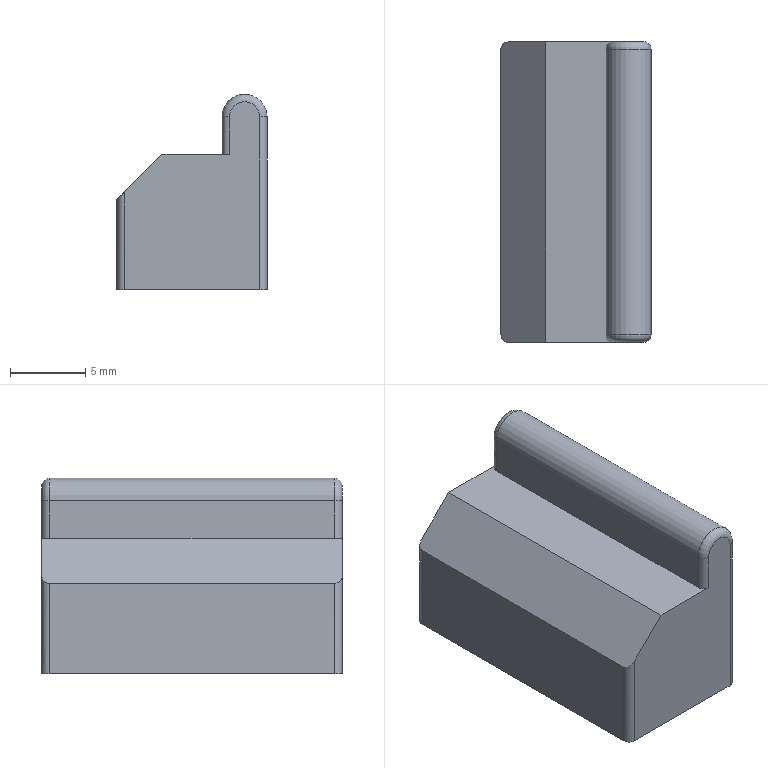Part | Mastercam | 1 solid | 28 faces | box 10 x 20 x 13 mm | volume 1837 mm3 | cylinder 13 | plane 9 | cone 4 | torus 2 | commonest cylinder face diameters 1 x6 2.5 x4 1.6 x2 3 x1
STEP:
#1=CARTESIAN_POINT('',(0.,0.,0.));
#2=DIRECTION('',(0.,0.,1.));
#3=DIRECTION('',(1.,0.,0.));
#4=AXIS2_PLACEMENT_3D('',#1,#2,#3);
#5=CARTESIAN_POINT('',(-8.,10.,0.));
#6=VERTEX_POINT('',#5);
#7=CARTESIAN_POINT('',(1.,10.,0.));
#8=VERTEX_POINT('',#7);
#9=CARTESIAN_POINT('',(-1.5,10.,0.));
#10=DIRECTION('',(1.,0.,0.));
#11=VECTOR('',#10,1.);
#12=LINE('',#9,#11);
#13=EDGE_CURVE('',#6,#8,#12,.T.);
#14=ORIENTED_EDGE('',*,*,#13,.T.);
#15=CARTESIAN_POINT('',(1.5,9.5,0.));
#16=VERTEX_POINT('',#15);
#17=CARTESIAN_POINT('',(1.,9.5,0.));
#18=DIRECTION('',(0.,0.,1.));
#19=DIRECTION('',(1.,0.,0.));
#20=AXIS2_PLACEMENT_3D('',#17,#18,#19);
#21=CIRCLE('',#20,0.5);
#22=EDGE_CURVE('',#16,#8,#21,.T.);
#23=ORIENTED_EDGE('',*,*,#22,.F.);
#24=CARTESIAN_POINT('',(1.5,-9.5,0.));
#25=VERTEX_POINT('',#24);
#26=CARTESIAN_POINT('',(1.5,-10.,0.));
#27=DIRECTION('',(0.,-1.,0.));
#28=VECTOR('',#27,1.);
#29=LINE('',#26,#28);
#30=EDGE_CURVE('',#16,#25,#29,.T.);
#31=ORIENTED_EDGE('',*,*,#30,.T.);
#32=CARTESIAN_POINT('',(1.,-10.,0.));
#33=VERTEX_POINT('',#32);
#34=CARTESIAN_POINT('',(1.,-9.5,0.));
#35=DIRECTION('',(0.,0.,1.));
#36=DIRECTION('',(1.,0.,0.));
#37=AXIS2_PLACEMENT_3D('',#34,#35,#36);
#38=CIRCLE('',#37,0.5);
#39=EDGE_CURVE('',#33,#25,#38,.T.);
#40=ORIENTED_EDGE('',*,*,#39,.F.);
#41=CARTESIAN_POINT('',(-8.,-10.,0.));
#42=VERTEX_POINT('',#41);
#43=CARTESIAN_POINT('',(-1.5,-10.,0.));
#44=DIRECTION('',(-1.,0.,0.));
#45=VECTOR('',#44,1.);
#46=LINE('',#43,#45);
#47=EDGE_CURVE('',#33,#42,#46,.T.);
#48=ORIENTED_EDGE('',*,*,#47,.T.);
#49=CARTESIAN_POINT('',(-8.5,-9.5,0.));
#50=VERTEX_POINT('',#49);
#51=CARTESIAN_POINT('',(-8.,-9.5,0.));
#52=DIRECTION('',(0.,0.,1.));
#53=DIRECTION('',(1.,0.,0.));
#54=AXIS2_PLACEMENT_3D('',#51,#52,#53);
#55=CIRCLE('',#54,0.5);
#56=EDGE_CURVE('',#50,#42,#55,.T.);
#57=ORIENTED_EDGE('',*,*,#56,.F.);
#58=CARTESIAN_POINT('',(-8.5,9.5,0.));
#59=VERTEX_POINT('',#58);
#60=CARTESIAN_POINT('',(-8.5,-10.,0.));
#61=DIRECTION('',(0.,-1.,0.));
#62=VECTOR('',#61,1.);
#63=LINE('',#60,#62);
#64=EDGE_CURVE('',#59,#50,#63,.T.);
#65=ORIENTED_EDGE('',*,*,#64,.F.);
#66=CARTESIAN_POINT('',(-8.,9.5,0.));
#67=DIRECTION('',(0.,0.,1.));
#68=DIRECTION('',(1.,0.,0.));
#69=AXIS2_PLACEMENT_3D('',#66,#67,#68);
#70=CIRCLE('',#69,0.5);
#71=EDGE_CURVE('',#6,#59,#70,.T.);
#72=ORIENTED_EDGE('',*,*,#71,.F.);
#73=EDGE_LOOP('',(#14,#23,#31,#40,#48,#57,#65,#72));
#74=FACE_OUTER_BOUND('',#73,.T.);
#75=CARTESIAN_POINT('',(-5.75,5.,0.));
#76=VERTEX_POINT('',#75);
#77=CARTESIAN_POINT('',(-3.25,5.,0.));
#78=VERTEX_POINT('',#77);
#79=CARTESIAN_POINT('',(-4.5,5.,0.));
#80=DIRECTION('',(0.,0.,1.));
#81=DIRECTION('',(-1.,0.,0.));
#82=AXIS2_PLACEMENT_3D('',#79,#80,#81);
#83=CIRCLE('',#82,1.25);
#84=EDGE_CURVE('',#76,#78,#83,.T.);
#85=ORIENTED_EDGE('',*,*,#84,.T.);
#86=CARTESIAN_POINT('',(-4.5,5.,0.));
#87=DIRECTION('',(0.,0.,1.));
#88=DIRECTION('',(-1.,0.,0.));
#89=AXIS2_PLACEMENT_3D('',#86,#87,#88);
#90=CIRCLE('',#89,1.25);
#91=EDGE_CURVE('',#78,#76,#90,.T.);
#92=ORIENTED_EDGE('',*,*,#91,.T.);
#93=EDGE_LOOP('',(#85,#92));
#94=FACE_BOUND('',#93,.T.);
#95=CARTESIAN_POINT('',(-5.75,-5.,0.));
#96=VERTEX_POINT('',#95);
#97=CARTESIAN_POINT('',(-3.25,-5.,0.));
#98=VERTEX_POINT('',#97);
#99=CARTESIAN_POINT('',(-4.5,-5.,0.));
#100=DIRECTION('',(0.,0.,1.));
#101=DIRECTION('',(-1.,0.,0.));
#102=AXIS2_PLACEMENT_3D('',#99,#100,#101);
#103=CIRCLE('',#102,1.25);
#104=EDGE_CURVE('',#96,#98,#103,.T.);
#105=ORIENTED_EDGE('',*,*,#104,.T.);
#106=CARTESIAN_POINT('',(-4.5,-5.,0.));
#107=DIRECTION('',(0.,0.,1.));
#108=DIRECTION('',(-1.,0.,0.));
#109=AXIS2_PLACEMENT_3D('',#106,#107,#108);
#110=CIRCLE('',#109,1.25);
#111=EDGE_CURVE('',#98,#96,#110,.T.);
#112=ORIENTED_EDGE('',*,*,#111,.T.);
#113=EDGE_LOOP('',(#105,#112));
#114=FACE_BOUND('',#113,.T.);
#115=CARTESIAN_POINT('',(0.,0.,0.));
#116=DIRECTION('',(0.,0.,1.));
#117=DIRECTION('',(1.,0.,0.));
#118=AXIS2_PLACEMENT_3D('',#115,#116,#117);
#119=PLANE('',#118);
#120=ADVANCED_FACE('',(#74,#94,#114),#119,.F.);
#121=CARTESIAN_POINT('',(-1.5,9.5,9.));
#122=VERTEX_POINT('',#121);
#123=CARTESIAN_POINT('',(-1.5,-9.5,9.));
#124=VERTEX_POINT('',#123);
#125=CARTESIAN_POINT('',(-1.5,-10.,9.));
#126=DIRECTION('',(0.,-1.,0.));
#127=VECTOR('',#126,1.);
#128=LINE('',#125,#127);
#129=EDGE_CURVE('',#122,#124,#128,.T.);
#130=ORIENTED_EDGE('',*,*,#129,.T.);
#131=CARTESIAN_POINT('',(-1.5,-9.5,11.5));
#132=VERTEX_POINT('',#131);
#133=CARTESIAN_POINT('',(-1.5,-9.5,13.));
#134=DIRECTION('',(0.,0.,-1.));
#135=VECTOR('',#134,1.);
#136=LINE('',#133,#135);
#137=EDGE_CURVE('',#132,#124,#136,.T.);
#138=ORIENTED_EDGE('',*,*,#137,.F.);
#139=CARTESIAN_POINT('',(-1.5,9.5,11.5));
#140=VERTEX_POINT('',#139);
#141=CARTESIAN_POINT('',(-1.5,-10.,11.5));
#142=DIRECTION('',(0.,-1.,0.));
#143=VECTOR('',#142,1.);
#144=LINE('',#141,#143);
#145=EDGE_CURVE('',#140,#132,#144,.T.);
#146=ORIENTED_EDGE('',*,*,#145,.F.);
#147=CARTESIAN_POINT('',(-1.5,9.5,13.));
#148=DIRECTION('',(0.,0.,1.));
#149=VECTOR('',#148,1.);
#150=LINE('',#147,#149);
#151=EDGE_CURVE('',#122,#140,#150,.T.);
#152=ORIENTED_EDGE('',*,*,#151,.F.);
#153=EDGE_LOOP('',(#130,#138,#146,#152));
#154=FACE_OUTER_BOUND('',#153,.T.);
#155=CARTESIAN_POINT('',(-1.5,-10.,13.));
#156=DIRECTION('',(1.,0.,0.));
#157=DIRECTION('',(0.,-1.,0.));
#158=AXIS2_PLACEMENT_3D('',#155,#156,#157);
#159=PLANE('',#158);
#160=ADVANCED_FACE('',(#154),#159,.F.);
#161=CARTESIAN_POINT('',(1.5,-9.5,11.5));
#162=VERTEX_POINT('',#161);
#163=CARTESIAN_POINT('',(1.5,9.5,11.5));
#164=VERTEX_POINT('',#163);
#165=CARTESIAN_POINT('',(1.5,10.,11.5));
#166=DIRECTION('',(0.,1.,0.));
#167=VECTOR('',#166,1.);
#168=LINE('',#165,#167);
#169=EDGE_CURVE('',#162,#164,#168,.T.);
#170=ORIENTED_EDGE('',*,*,#169,.F.);
#171=CARTESIAN_POINT('',(1.5,-9.5,13.));
#172=DIRECTION('',(0.,0.,1.));
#173=VECTOR('',#172,1.);
#174=LINE('',#171,#173);
#175=EDGE_CURVE('',#25,#162,#174,.T.);
#176=ORIENTED_EDGE('',*,*,#175,.F.);
#177=ORIENTED_EDGE('',*,*,#30,.F.);
#178=CARTESIAN_POINT('',(1.5,9.5,13.));
#179=DIRECTION('',(0.,0.,-1.));
#180=VECTOR('',#179,1.);
#181=LINE('',#178,#180);
#182=EDGE_CURVE('',#164,#16,#181,.T.);
#183=ORIENTED_EDGE('',*,*,#182,.F.);
#184=EDGE_LOOP('',(#170,#176,#177,#183));
#185=FACE_OUTER_BOUND('',#184,.T.);
#186=CARTESIAN_POINT('',(1.5,-10.,13.));
#187=DIRECTION('',(-1.,0.,0.));
#188=DIRECTION('',(0.,1.,0.));
#189=AXIS2_PLACEMENT_3D('',#186,#187,#188);
#190=PLANE('',#189);
#191=ADVANCED_FACE('',(#185),#190,.F.);
#192=CARTESIAN_POINT('',(-8.,-10.,6.5));
#193=VERTEX_POINT('',#192);
#194=CARTESIAN_POINT('',(-8.,-10.,9.));
#195=DIRECTION('',(0.,0.,1.));
#196=VECTOR('',#195,1.);
#197=LINE('',#194,#196);
#198=EDGE_CURVE('',#42,#193,#197,.T.);
#199=ORIENTED_EDGE('',*,*,#198,.F.);
#200=ORIENTED_EDGE('',*,*,#47,.F.);
#201=CARTESIAN_POINT('',(1.,-10.,11.5));
#202=VERTEX_POINT('',#201);
#203=CARTESIAN_POINT('',(1.,-10.,13.));
#204=DIRECTION('',(0.,0.,-1.));
#205=VECTOR('',#204,1.);
#206=LINE('',#203,#205);
#207=EDGE_CURVE('',#202,#33,#206,.T.);
#208=ORIENTED_EDGE('',*,*,#207,.F.);
#209=CARTESIAN_POINT('',(-1.,-10.,11.5));
#210=VERTEX_POINT('',#209);
#211=CARTESIAN_POINT('',(0.,-10.,11.5));
#212=DIRECTION('',(0.,1.,0.));
#213=DIRECTION('',(0.,0.,-1.));
#214=AXIS2_PLACEMENT_3D('',#211,#212,#213);
#215=CIRCLE('',#214,1.);
#216=EDGE_CURVE('',#210,#202,#215,.T.);
#217=ORIENTED_EDGE('',*,*,#216,.F.);
#218=CARTESIAN_POINT('',(-1.,-10.,9.));
#219=VERTEX_POINT('',#218);
#220=CARTESIAN_POINT('',(-1.,-10.,13.));
#221=DIRECTION('',(0.,0.,1.));
#222=VECTOR('',#221,1.);
#223=LINE('',#220,#222);
#224=EDGE_CURVE('',#219,#210,#223,.T.);
#225=ORIENTED_EDGE('',*,*,#224,.F.);
#226=CARTESIAN_POINT('',(-5.5,-10.,9.));
#227=VERTEX_POINT('',#226);
#228=CARTESIAN_POINT('',(1.5,-10.,9.));
#229=DIRECTION('',(1.,0.,0.));
#230=VECTOR('',#229,1.);
#231=LINE('',#228,#230);
#232=EDGE_CURVE('',#227,#219,#231,.T.);
#233=ORIENTED_EDGE('',*,*,#232,.F.);
#234=CARTESIAN_POINT('',(-8.5,-10.,6.));
#235=DIRECTION('',(0.7071,0.,0.7071));
#236=VECTOR('',#235,1.);
#237=LINE('',#234,#236);
#238=EDGE_CURVE('',#193,#227,#237,.T.);
#239=ORIENTED_EDGE('',*,*,#238,.F.);
#240=EDGE_LOOP('',(#199,#200,#208,#217,#225,#233,#239));
#241=FACE_OUTER_BOUND('',#240,.T.);
#242=CARTESIAN_POINT('',(-1.5,-10.,13.));
#243=DIRECTION('',(0.,1.,0.));
#244=DIRECTION('',(0.,0.,-1.));
#245=AXIS2_PLACEMENT_3D('',#242,#243,#244);
#246=PLANE('',#245);
#247=ADVANCED_FACE('',(#241),#246,.F.);
#248=CARTESIAN_POINT('',(-1.,10.,9.));
#249=VERTEX_POINT('',#248);
#250=CARTESIAN_POINT('',(-5.5,10.,9.));
#251=VERTEX_POINT('',#250);
#252=CARTESIAN_POINT('',(1.5,10.,9.));
#253=DIRECTION('',(-1.,0.,0.));
#254=VECTOR('',#253,1.);
#255=LINE('',#252,#254);
#256=EDGE_CURVE('',#249,#251,#255,.T.);
#257=ORIENTED_EDGE('',*,*,#256,.F.);
#258=CARTESIAN_POINT('',(-1.,10.,11.5));
#259=VERTEX_POINT('',#258);
#260=CARTESIAN_POINT('',(-1.,10.,13.));
#261=DIRECTION('',(0.,0.,-1.));
#262=VECTOR('',#261,1.);
#263=LINE('',#260,#262);
#264=EDGE_CURVE('',#259,#249,#263,.T.);
#265=ORIENTED_EDGE('',*,*,#264,.F.);
#266=CARTESIAN_POINT('',(1.,10.,11.5));
#267=VERTEX_POINT('',#266);
#268=CARTESIAN_POINT('',(0.,10.,11.5));
#269=DIRECTION('',(0.,-1.,0.));
#270=DIRECTION('',(0.,0.,1.));
#271=AXIS2_PLACEMENT_3D('',#268,#269,#270);
#272=CIRCLE('',#271,1.);
#273=EDGE_CURVE('',#267,#259,#272,.T.);
#274=ORIENTED_EDGE('',*,*,#273,.F.);
#275=CARTESIAN_POINT('',(1.,10.,13.));
#276=DIRECTION('',(0.,0.,1.));
#277=VECTOR('',#276,1.);
#278=LINE('',#275,#277);
#279=EDGE_CURVE('',#8,#267,#278,.T.);
#280=ORIENTED_EDGE('',*,*,#279,.F.);
#281=ORIENTED_EDGE('',*,*,#13,.F.);
#282=CARTESIAN_POINT('',(-8.,10.,6.5));
#283=VERTEX_POINT('',#282);
#284=CARTESIAN_POINT('',(-8.,10.,0.));
#285=DIRECTION('',(0.,0.,-1.));
#286=VECTOR('',#285,1.);
#287=LINE('',#284,#286);
#288=EDGE_CURVE('',#283,#6,#287,.T.);
#289=ORIENTED_EDGE('',*,*,#288,.F.);
#290=CARTESIAN_POINT('',(-8.5,10.,6.));
#291=DIRECTION('',(-0.7071,0.,-0.7071));
#292=VECTOR('',#291,1.);
#293=LINE('',#290,#292);
#294=EDGE_CURVE('',#251,#283,#293,.T.);
#295=ORIENTED_EDGE('',*,*,#294,.F.);
#296=EDGE_LOOP('',(#257,#265,#274,#280,#281,#289,#295));
#297=FACE_OUTER_BOUND('',#296,.T.);
#298=CARTESIAN_POINT('',(0.,10.,10.7));
#299=VERTEX_POINT('',#298);
#300=CARTESIAN_POINT('',(0.,10.,12.3));
#301=VERTEX_POINT('',#300);
#302=CARTESIAN_POINT('',(0.,10.,11.5));
#303=DIRECTION('',(0.,-1.,0.));
#304=DIRECTION('',(0.,0.,-1.));
#305=AXIS2_PLACEMENT_3D('',#302,#303,#304);
#306=CIRCLE('',#305,0.8);
#307=EDGE_CURVE('',#299,#301,#306,.T.);
#308=ORIENTED_EDGE('',*,*,#307,.T.);
#309=CARTESIAN_POINT('',(0.,10.,11.5));
#310=DIRECTION('',(0.,-1.,0.));
#311=DIRECTION('',(0.,0.,-1.));
#312=AXIS2_PLACEMENT_3D('',#309,#310,#311);
#313=CIRCLE('',#312,0.8);
#314=EDGE_CURVE('',#301,#299,#313,.T.);
#315=ORIENTED_EDGE('',*,*,#314,.T.);
#316=EDGE_LOOP('',(#308,#315));
#317=FACE_BOUND('',#316,.T.);
#318=CARTESIAN_POINT('',(-1.5,10.,13.));
#319=DIRECTION('',(0.,-1.,0.));
#320=DIRECTION('',(0.,0.,1.));
#321=AXIS2_PLACEMENT_3D('',#318,#319,#320);
#322=PLANE('',#321);
#323=ADVANCED_FACE('',(#297,#317),#322,.F.);
#324=ORIENTED_EDGE('',*,*,#145,.T.);
#325=CARTESIAN_POINT('',(0.,-9.5,11.5));
#326=DIRECTION('',(0.,-1.,0.));
#327=DIRECTION('',(0.,0.,-1.));
#328=AXIS2_PLACEMENT_3D('',#325,#326,#327);
#329=CIRCLE('',#328,1.5);
#330=EDGE_CURVE('',#162,#132,#329,.T.);
#331=ORIENTED_EDGE('',*,*,#330,.F.);
#332=ORIENTED_EDGE('',*,*,#169,.T.);
#333=CARTESIAN_POINT('',(0.,9.5,11.5));
#334=DIRECTION('',(0.,1.,0.));
#335=DIRECTION('',(0.,0.,1.));
#336=AXIS2_PLACEMENT_3D('',#333,#334,#335);
#337=CIRCLE('',#336,1.5);
#338=EDGE_CURVE('',#140,#164,#337,.T.);
#339=ORIENTED_EDGE('',*,*,#338,.F.);
#340=EDGE_LOOP('',(#324,#331,#332,#339));
#341=FACE_OUTER_BOUND('',#340,.T.);
#342=CARTESIAN_POINT('',(0.,0.,11.5));
#343=DIRECTION('',(0.,-1.,0.));
#344=DIRECTION('',(0.,0.,-1.));
#345=AXIS2_PLACEMENT_3D('',#342,#343,#344);
#346=CYLINDRICAL_SURFACE('',#345,1.5);
#347=ADVANCED_FACE('',(#341),#346,.T.);
#348=CARTESIAN_POINT('',(0.,-5.,12.3));
#349=VERTEX_POINT('',#348);
#350=CARTESIAN_POINT('',(0.,-5.,12.3));
#351=DIRECTION('',(0.,1.,0.));
#352=VECTOR('',#351,1.);
#353=LINE('',#350,#352);
#354=EDGE_CURVE('',#349,#301,#353,.T.);
#355=ORIENTED_EDGE('',*,*,#354,.T.);
#356=ORIENTED_EDGE('',*,*,#307,.F.);
#357=CARTESIAN_POINT('',(0.,-5.,10.7));
#358=VERTEX_POINT('',#357);
#359=CARTESIAN_POINT('',(0.,-5.,10.7));
#360=DIRECTION('',(0.,1.,0.));
#361=VECTOR('',#360,1.);
#362=LINE('',#359,#361);
#363=EDGE_CURVE('',#358,#299,#362,.T.);
#364=ORIENTED_EDGE('',*,*,#363,.F.);
#365=CARTESIAN_POINT('',(0.,-5.,11.5));
#366=DIRECTION('',(0.,-1.,0.));
#367=DIRECTION('',(0.,0.,-1.));
#368=AXIS2_PLACEMENT_3D('',#365,#366,#367);
#369=CIRCLE('',#368,0.8);
#370=EDGE_CURVE('',#358,#349,#369,.T.);
#371=ORIENTED_EDGE('',*,*,#370,.T.);
#372=EDGE_LOOP('',(#355,#356,#364,#371));
#373=FACE_OUTER_BOUND('',#372,.T.);
#374=CARTESIAN_POINT('',(0.,-5.,11.5));
#375=DIRECTION('',(0.,1.,0.));
#376=DIRECTION('',(-1.,0.,0.));
#377=AXIS2_PLACEMENT_3D('',#374,#375,#376);
#378=CYLINDRICAL_SURFACE('',#377,0.8);
#379=ADVANCED_FACE('',(#373),#378,.F.);
#380=CARTESIAN_POINT('',(0.,-5.,11.5));
#381=DIRECTION('',(0.,-1.,0.));
#382=DIRECTION('',(0.,0.,-1.));
#383=AXIS2_PLACEMENT_3D('',#380,#381,#382);
#384=CIRCLE('',#383,0.8);
#385=EDGE_CURVE('',#349,#358,#384,.T.);
#386=ORIENTED_EDGE('',*,*,#385,.F.);
#387=ORIENTED_EDGE('',*,*,#370,.F.);
#388=EDGE_LOOP('',(#386,#387));
#389=FACE_OUTER_BOUND('',#388,.T.);
#390=CARTESIAN_POINT('',(0.,-5.,11.5));
#391=DIRECTION('',(0.,1.,0.));
#392=DIRECTION('',(0.,0.,-1.));
#393=AXIS2_PLACEMENT_3D('',#390,#391,#392);
#394=PLANE('',#393);
#395=ADVANCED_FACE('',(#389),#394,.T.);
#396=ORIENTED_EDGE('',*,*,#232,.T.);
#397=CARTESIAN_POINT('',(-1.,-9.5,9.));
#398=DIRECTION('',(0.,0.,1.));
#399=DIRECTION('',(-1.,0.,0.));
#400=AXIS2_PLACEMENT_3D('',#397,#398,#399);
#401=CIRCLE('',#400,0.5);
#402=EDGE_CURVE('',#124,#219,#401,.T.);
#403=ORIENTED_EDGE('',*,*,#402,.F.);
#404=ORIENTED_EDGE('',*,*,#129,.F.);
#405=CARTESIAN_POINT('',(-1.,9.5,9.));
#406=DIRECTION('',(0.,0.,1.));
#407=DIRECTION('',(-1.,0.,0.));
#408=AXIS2_PLACEMENT_3D('',#405,#406,#407);
#409=CIRCLE('',#408,0.5);
#410=EDGE_CURVE('',#249,#122,#409,.T.);
#411=ORIENTED_EDGE('',*,*,#410,.F.);
#412=ORIENTED_EDGE('',*,*,#256,.T.);
#413=CARTESIAN_POINT('',(-5.5,9.5,9.));
#414=DIRECTION('',(0.,1.,0.));
#415=VECTOR('',#414,1.);
#416=LINE('',#413,#415);
#417=EDGE_CURVE('',#227,#251,#416,.T.);
#418=ORIENTED_EDGE('',*,*,#417,.F.);
#419=EDGE_LOOP('',(#396,#403,#404,#411,#412,#418));
#420=FACE_OUTER_BOUND('',#419,.T.);
#421=CARTESIAN_POINT('',(0.,0.,9.));
#422=DIRECTION('',(0.,0.,-1.));
#423=DIRECTION('',(-1.,0.,0.));
#424=AXIS2_PLACEMENT_3D('',#421,#422,#423);
#425=PLANE('',#424);
#426=ADVANCED_FACE('',(#420),#425,.F.);
#427=CARTESIAN_POINT('',(-8.5,9.5,6.));
#428=VERTEX_POINT('',#427);
#429=CARTESIAN_POINT('',(-8.5,9.5,9.));
#430=DIRECTION('',(0.,0.,1.));
#431=VECTOR('',#430,1.);
#432=LINE('',#429,#431);
#433=EDGE_CURVE('',#59,#428,#432,.T.);
#434=ORIENTED_EDGE('',*,*,#433,.F.);
#435=ORIENTED_EDGE('',*,*,#64,.T.);
#436=CARTESIAN_POINT('',(-8.5,-9.5,6.));
#437=VERTEX_POINT('',#436);
#438=CARTESIAN_POINT('',(-8.5,-9.5,0.));
#439=DIRECTION('',(0.,0.,-1.));
#440=VECTOR('',#439,1.);
#441=LINE('',#438,#440);
#442=EDGE_CURVE('',#437,#50,#441,.T.);
#443=ORIENTED_EDGE('',*,*,#442,.F.);
#444=CARTESIAN_POINT('',(-8.5,-9.5,6.));
#445=DIRECTION('',(0.,-1.,0.));
#446=VECTOR('',#445,1.);
#447=LINE('',#444,#446);
#448=EDGE_CURVE('',#428,#437,#447,.T.);
#449=ORIENTED_EDGE('',*,*,#448,.F.);
#450=EDGE_LOOP('',(#434,#435,#443,#449));
#451=FACE_OUTER_BOUND('',#450,.T.);
#452=CARTESIAN_POINT('',(-8.5,-10.,9.));
#453=DIRECTION('',(-1.,0.,0.));
#454=DIRECTION('',(0.,1.,0.));
#455=AXIS2_PLACEMENT_3D('',#452,#453,#454);
#456=PLANE('',#455);
#457=ADVANCED_FACE('',(#451),#456,.T.);
#458=CARTESIAN_POINT('',(-4.5,5.,6.751));
#459=VERTEX_POINT('',#458);
#460=CARTESIAN_POINT('',(-3.25,5.,6.));
#461=VERTEX_POINT('',#460);
#462=CARTESIAN_POINT('',(-4.5,5.,6.751));
#463=DIRECTION('',(0.8572,0.,-0.515));
#464=VECTOR('',#463,1.);
#465=LINE('',#462,#464);
#466=EDGE_CURVE('',#459,#461,#465,.T.);
#467=ORIENTED_EDGE('',*,*,#466,.T.);
#468=CARTESIAN_POINT('',(-5.75,5.,6.));
#469=VERTEX_POINT('',#468);
#470=CARTESIAN_POINT('',(-4.5,5.,6.));
#471=DIRECTION('',(0.,0.,1.));
#472=DIRECTION('',(-1.,0.,0.));
#473=AXIS2_PLACEMENT_3D('',#470,#471,#472);
#474=CIRCLE('',#473,1.25);
#475=EDGE_CURVE('',#469,#461,#474,.T.);
#476=ORIENTED_EDGE('',*,*,#475,.F.);
#477=CARTESIAN_POINT('',(-4.5,5.,6.751));
#478=DIRECTION('',(-0.8572,0.,-0.515));
#479=VECTOR('',#478,1.);
#480=LINE('',#477,#479);
#481=EDGE_CURVE('',#459,#469,#480,.T.);
#482=ORIENTED_EDGE('',*,*,#481,.F.);
#483=EDGE_LOOP('',(#467,#476,#482));
#484=FACE_OUTER_BOUND('',#483,.T.);
#485=CARTESIAN_POINT('',(-4.5,5.,6.));
#486=DIRECTION('',(0.,0.,-1.));
#487=DIRECTION('',(0.,1.,0.));
#488=AXIS2_PLACEMENT_3D('',#485,#486,#487);
#489=CONICAL_SURFACE('',#488,1.25,1.03);
#490=ADVANCED_FACE('',(#484),#489,.F.);
#491=CARTESIAN_POINT('',(-3.25,5.,6.));
#492=DIRECTION('',(0.,0.,-1.));
#493=VECTOR('',#492,1.);
#494=LINE('',#491,#493);
#495=EDGE_CURVE('',#461,#78,#494,.T.);
#496=ORIENTED_EDGE('',*,*,#495,.T.);
#497=ORIENTED_EDGE('',*,*,#84,.F.);
#498=CARTESIAN_POINT('',(-5.75,5.,6.));
#499=DIRECTION('',(0.,0.,-1.));
#500=VECTOR('',#499,1.);
#501=LINE('',#498,#500);
#502=EDGE_CURVE('',#469,#76,#501,.T.);
#503=ORIENTED_EDGE('',*,*,#502,.F.);
#504=ORIENTED_EDGE('',*,*,#475,.T.);
#505=EDGE_LOOP('',(#496,#497,#503,#504));
#506=FACE_OUTER_BOUND('',#505,.T.);
#507=CARTESIAN_POINT('',(-4.5,5.,0.));
#508=DIRECTION('',(0.,0.,-1.));
#509=DIRECTION('',(0.,1.,0.));
#510=AXIS2_PLACEMENT_3D('',#507,#508,#509);
#511=CYLINDRICAL_SURFACE('',#510,1.25);
#512=ADVANCED_FACE('',(#506),#511,.F.);
#513=CARTESIAN_POINT('',(-4.5,-5.,6.751));
#514=VERTEX_POINT('',#513);
#515=CARTESIAN_POINT('',(-3.25,-5.,6.));
#516=VERTEX_POINT('',#515);
#517=CARTESIAN_POINT('',(-4.5,-5.,6.751));
#518=DIRECTION('',(0.8572,0.,-0.515));
#519=VECTOR('',#518,1.);
#520=LINE('',#517,#519);
#521=EDGE_CURVE('',#514,#516,#520,.T.);
#522=ORIENTED_EDGE('',*,*,#521,.T.);
#523=CARTESIAN_POINT('',(-5.75,-5.,6.));
#524=VERTEX_POINT('',#523);
#525=CARTESIAN_POINT('',(-4.5,-5.,6.));
#526=DIRECTION('',(0.,0.,1.));
#527=DIRECTION('',(-1.,0.,0.));
#528=AXIS2_PLACEMENT_3D('',#525,#526,#527);
#529=CIRCLE('',#528,1.25);
#530=EDGE_CURVE('',#524,#516,#529,.T.);
#531=ORIENTED_EDGE('',*,*,#530,.F.);
#532=CARTESIAN_POINT('',(-4.5,-5.,6.751));
#533=DIRECTION('',(-0.8572,0.,-0.515));
#534=VECTOR('',#533,1.);
#535=LINE('',#532,#534);
#536=EDGE_CURVE('',#514,#524,#535,.T.);
#537=ORIENTED_EDGE('',*,*,#536,.F.);
#538=EDGE_LOOP('',(#522,#531,#537));
#539=FACE_OUTER_BOUND('',#538,.T.);
#540=CARTESIAN_POINT('',(-4.5,-5.,6.));
#541=DIRECTION('',(0.,0.,-1.));
#542=DIRECTION('',(0.,1.,0.));
#543=AXIS2_PLACEMENT_3D('',#540,#541,#542);
#544=CONICAL_SURFACE('',#543,1.25,1.03);
#545=ADVANCED_FACE('',(#539),#544,.F.);
#546=CARTESIAN_POINT('',(-3.25,-5.,6.));
#547=DIRECTION('',(0.,0.,-1.));
#548=VECTOR('',#547,1.);
#549=LINE('',#546,#548);
#550=EDGE_CURVE('',#516,#98,#549,.T.);
#551=ORIENTED_EDGE('',*,*,#550,.T.);
#552=ORIENTED_EDGE('',*,*,#104,.F.);
#553=CARTESIAN_POINT('',(-5.75,-5.,6.));
#554=DIRECTION('',(0.,0.,-1.));
#555=VECTOR('',#554,1.);
#556=LINE('',#553,#555);
#557=EDGE_CURVE('',#524,#96,#556,.T.);
#558=ORIENTED_EDGE('',*,*,#557,.F.);
#559=ORIENTED_EDGE('',*,*,#530,.T.);
#560=EDGE_LOOP('',(#551,#552,#558,#559));
#561=FACE_OUTER_BOUND('',#560,.T.);
#562=CARTESIAN_POINT('',(-4.5,-5.,0.));
#563=DIRECTION('',(0.,0.,-1.));
#564=DIRECTION('',(0.,1.,0.));
#565=AXIS2_PLACEMENT_3D('',#562,#563,#564);
#566=CYLINDRICAL_SURFACE('',#565,1.25);
#567=ADVANCED_FACE('',(#561),#566,.F.);
#568=ORIENTED_EDGE('',*,*,#22,.T.);
#569=ORIENTED_EDGE('',*,*,#279,.T.);
#570=CARTESIAN_POINT('',(1.,9.5,11.5));
#571=DIRECTION('',(0.,0.,-1.));
#572=DIRECTION('',(1.,0.,0.));
#573=AXIS2_PLACEMENT_3D('',#570,#571,#572);
#574=CIRCLE('',#573,0.5);
#575=EDGE_CURVE('',#267,#164,#574,.T.);
#576=ORIENTED_EDGE('',*,*,#575,.T.);
#577=ORIENTED_EDGE('',*,*,#182,.T.);
#578=EDGE_LOOP('',(#568,#569,#576,#577));
#579=FACE_OUTER_BOUND('',#578,.T.);
#580=CARTESIAN_POINT('',(1.,9.5,13.));
#581=DIRECTION('',(0.,0.,-1.));
#582=DIRECTION('',(-0.7071,-0.7071,0.));
#583=AXIS2_PLACEMENT_3D('',#580,#581,#582);
#584=CYLINDRICAL_SURFACE('',#583,0.5);
#585=ADVANCED_FACE('',(#579),#584,.T.);
#586=ORIENTED_EDGE('',*,*,#575,.F.);
#587=ORIENTED_EDGE('',*,*,#273,.T.);
#588=CARTESIAN_POINT('',(-1.,9.5,11.5));
#589=DIRECTION('',(0.,0.,1.));
#590=DIRECTION('',(-1.,0.,0.));
#591=AXIS2_PLACEMENT_3D('',#588,#589,#590);
#592=CIRCLE('',#591,0.5);
#593=EDGE_CURVE('',#259,#140,#592,.T.);
#594=ORIENTED_EDGE('',*,*,#593,.T.);
#595=ORIENTED_EDGE('',*,*,#338,.T.);
#596=EDGE_LOOP('',(#586,#587,#594,#595));
#597=FACE_OUTER_BOUND('',#596,.T.);
#598=CARTESIAN_POINT('',(0.,9.5,11.5));
#599=DIRECTION('',(0.,-1.,0.));
#600=DIRECTION('',(0.,0.,-1.));
#601=AXIS2_PLACEMENT_3D('',#598,#599,#600);
#602=TOROIDAL_SURFACE('',#601,1.,0.5);
#603=ADVANCED_FACE('',(#597),#602,.T.);
#604=ORIENTED_EDGE('',*,*,#593,.F.);
#605=ORIENTED_EDGE('',*,*,#264,.T.);
#606=ORIENTED_EDGE('',*,*,#410,.T.);
#607=ORIENTED_EDGE('',*,*,#151,.T.);
#608=EDGE_LOOP('',(#604,#605,#606,#607));
#609=FACE_OUTER_BOUND('',#608,.T.);
#610=CARTESIAN_POINT('',(-1.,9.5,13.));
#611=DIRECTION('',(0.,0.,-1.));
#612=DIRECTION('',(0.7071,-0.7071,0.));
#613=AXIS2_PLACEMENT_3D('',#610,#611,#612);
#614=CYLINDRICAL_SURFACE('',#613,0.5);
#615=ADVANCED_FACE('',(#609),#614,.T.);
#616=ORIENTED_EDGE('',*,*,#39,.T.);
#617=ORIENTED_EDGE('',*,*,#175,.T.);
#618=CARTESIAN_POINT('',(1.,-9.5,11.5));
#619=DIRECTION('',(0.,0.,-1.));
#620=DIRECTION('',(1.,0.,0.));
#621=AXIS2_PLACEMENT_3D('',#618,#619,#620);
#622=CIRCLE('',#621,0.5);
#623=EDGE_CURVE('',#162,#202,#622,.T.);
#624=ORIENTED_EDGE('',*,*,#623,.T.);
#625=ORIENTED_EDGE('',*,*,#207,.T.);
#626=EDGE_LOOP('',(#616,#617,#624,#625));
#627=FACE_OUTER_BOUND('',#626,.T.);
#628=CARTESIAN_POINT('',(1.,-9.5,13.));
#629=DIRECTION('',(0.,0.,-1.));
#630=DIRECTION('',(-0.7071,0.7071,0.));
#631=AXIS2_PLACEMENT_3D('',#628,#629,#630);
#632=CYLINDRICAL_SURFACE('',#631,0.5);
#633=ADVANCED_FACE('',(#627),#632,.T.);
#634=ORIENTED_EDGE('',*,*,#623,.F.);
#635=ORIENTED_EDGE('',*,*,#330,.T.);
#636=CARTESIAN_POINT('',(-1.,-9.5,11.5));
#637=DIRECTION('',(0.,0.,1.));
#638=DIRECTION('',(-1.,0.,0.));
#639=AXIS2_PLACEMENT_3D('',#636,#637,#638);
#640=CIRCLE('',#639,0.5);
#641=EDGE_CURVE('',#132,#210,#640,.T.);
#642=ORIENTED_EDGE('',*,*,#641,.T.);
#643=ORIENTED_EDGE('',*,*,#216,.T.);
#644=EDGE_LOOP('',(#634,#635,#642,#643));
#645=FACE_OUTER_BOUND('',#644,.T.);
#646=CARTESIAN_POINT('',(0.,-9.5,11.5));
#647=DIRECTION('',(0.,1.,0.));
#648=DIRECTION('',(0.,0.,-1.));
#649=AXIS2_PLACEMENT_3D('',#646,#647,#648);
#650=TOROIDAL_SURFACE('',#649,1.,0.5);
#651=ADVANCED_FACE('',(#645),#650,.T.);
#652=ORIENTED_EDGE('',*,*,#641,.F.);
#653=ORIENTED_EDGE('',*,*,#137,.T.);
#654=ORIENTED_EDGE('',*,*,#402,.T.);
#655=ORIENTED_EDGE('',*,*,#224,.T.);
#656=EDGE_LOOP('',(#652,#653,#654,#655));
#657=FACE_OUTER_BOUND('',#656,.T.);
#658=CARTESIAN_POINT('',(-1.,-9.5,13.));
#659=DIRECTION('',(0.,0.,-1.));
#660=DIRECTION('',(0.7071,0.7071,0.));
#661=AXIS2_PLACEMENT_3D('',#658,#659,#660);
#662=CYLINDRICAL_SURFACE('',#661,0.5);
#663=ADVANCED_FACE('',(#657),#662,.T.);
#664=ORIENTED_EDGE('',*,*,#288,.T.);
#665=ORIENTED_EDGE('',*,*,#71,.T.);
#666=ORIENTED_EDGE('',*,*,#433,.T.);
#667=CARTESIAN_POINT('',(-8.,9.5,6.5));
#668=DIRECTION('',(-0.7071,0.,0.7071));
#669=DIRECTION('',(0.7071,0.,0.7071));
#670=AXIS2_PLACEMENT_3D('',#667,#668,#669);
#671=ELLIPSE('',#670,0.7071,0.5);
#672=EDGE_CURVE('',#283,#428,#671,.T.);
#673=ORIENTED_EDGE('',*,*,#672,.F.);
#674=EDGE_LOOP('',(#664,#665,#666,#673));
#675=FACE_OUTER_BOUND('',#674,.T.);
#676=CARTESIAN_POINT('',(-8.,9.5,13.));
#677=DIRECTION('',(0.,0.,1.));
#678=DIRECTION('',(0.7071,-0.7071,0.));
#679=AXIS2_PLACEMENT_3D('',#676,#677,#678);
#680=CYLINDRICAL_SURFACE('',#679,0.5);
#681=ADVANCED_FACE('',(#675),#680,.T.);
#682=ORIENTED_EDGE('',*,*,#442,.T.);
#683=ORIENTED_EDGE('',*,*,#56,.T.);
#684=ORIENTED_EDGE('',*,*,#198,.T.);
#685=CARTESIAN_POINT('',(-8.,-9.5,6.5));
#686=DIRECTION('',(-0.7071,0.,0.7071));
#687=DIRECTION('',(0.7071,0.,0.7071));
#688=AXIS2_PLACEMENT_3D('',#685,#686,#687);
#689=ELLIPSE('',#688,0.7071,0.5);
#690=EDGE_CURVE('',#437,#193,#689,.T.);
#691=ORIENTED_EDGE('',*,*,#690,.F.);
#692=EDGE_LOOP('',(#682,#683,#684,#691));
#693=FACE_OUTER_BOUND('',#692,.T.);
#694=CARTESIAN_POINT('',(-8.,-9.5,9.));
#695=DIRECTION('',(0.,0.,1.));
#696=DIRECTION('',(0.7071,0.7071,0.));
#697=AXIS2_PLACEMENT_3D('',#694,#695,#696);
#698=CYLINDRICAL_SURFACE('',#697,0.5);
#699=ADVANCED_FACE('',(#693),#698,.T.);
#700=ORIENTED_EDGE('',*,*,#294,.T.);
#701=ORIENTED_EDGE('',*,*,#672,.T.);
#702=ORIENTED_EDGE('',*,*,#448,.T.);
#703=ORIENTED_EDGE('',*,*,#690,.T.);
#704=ORIENTED_EDGE('',*,*,#238,.T.);
#705=ORIENTED_EDGE('',*,*,#417,.T.);
#706=EDGE_LOOP('',(#700,#701,#702,#703,#704,#705));
#707=FACE_OUTER_BOUND('',#706,.T.);
#708=CARTESIAN_POINT('',(-8.5,-10.,6.));
#709=DIRECTION('',(-0.7071,0.,0.7071));
#710=DIRECTION('',(0.,1.,0.));
#711=AXIS2_PLACEMENT_3D('',#708,#709,#710);
#712=PLANE('',#711);
#713=ADVANCED_FACE('',(#707),#712,.T.);
#714=ORIENTED_EDGE('',*,*,#354,.F.);
#715=ORIENTED_EDGE('',*,*,#385,.T.);
#716=ORIENTED_EDGE('',*,*,#363,.T.);
#717=ORIENTED_EDGE('',*,*,#314,.F.);
#718=EDGE_LOOP('',(#714,#715,#716,#717));
#719=FACE_OUTER_BOUND('',#718,.T.);
#720=CARTESIAN_POINT('',(0.,-5.,11.5));
#721=DIRECTION('',(0.,1.,0.));
#722=DIRECTION('',(1.,0.,0.));
#723=AXIS2_PLACEMENT_3D('',#720,#721,#722);
#724=CYLINDRICAL_SURFACE('',#723,0.8);
#725=ADVANCED_FACE('',(#719),#724,.F.);
#726=ORIENTED_EDGE('',*,*,#481,.T.);
#727=CARTESIAN_POINT('',(-4.5,5.,6.));
#728=DIRECTION('',(0.,0.,1.));
#729=DIRECTION('',(-1.,0.,0.));
#730=AXIS2_PLACEMENT_3D('',#727,#728,#729);
#731=CIRCLE('',#730,1.25);
#732=EDGE_CURVE('',#461,#469,#731,.T.);
#733=ORIENTED_EDGE('',*,*,#732,.F.);
#734=ORIENTED_EDGE('',*,*,#466,.F.);
#735=EDGE_LOOP('',(#726,#733,#734));
#736=FACE_OUTER_BOUND('',#735,.T.);
#737=CARTESIAN_POINT('',(-4.5,5.,6.));
#738=DIRECTION('',(0.,0.,-1.));
#739=DIRECTION('',(0.,-1.,0.));
#740=AXIS2_PLACEMENT_3D('',#737,#738,#739);
#741=CONICAL_SURFACE('',#740,1.25,1.03);
#742=ADVANCED_FACE('',(#736),#741,.F.);
#743=ORIENTED_EDGE('',*,*,#495,.F.);
#744=ORIENTED_EDGE('',*,*,#732,.T.);
#745=ORIENTED_EDGE('',*,*,#502,.T.);
#746=ORIENTED_EDGE('',*,*,#91,.F.);
#747=EDGE_LOOP('',(#743,#744,#745,#746));
#748=FACE_OUTER_BOUND('',#747,.T.);
#749=CARTESIAN_POINT('',(-4.5,5.,0.));
#750=DIRECTION('',(0.,0.,-1.));
#751=DIRECTION('',(0.,-1.,0.));
#752=AXIS2_PLACEMENT_3D('',#749,#750,#751);
#753=CYLINDRICAL_SURFACE('',#752,1.25);
#754=ADVANCED_FACE('',(#748),#753,.F.);
#755=ORIENTED_EDGE('',*,*,#536,.T.);
#756=CARTESIAN_POINT('',(-4.5,-5.,6.));
#757=DIRECTION('',(0.,0.,1.));
#758=DIRECTION('',(-1.,0.,0.));
#759=AXIS2_PLACEMENT_3D('',#756,#757,#758);
#760=CIRCLE('',#759,1.25);
#761=EDGE_CURVE('',#516,#524,#760,.T.);
#762=ORIENTED_EDGE('',*,*,#761,.F.);
#763=ORIENTED_EDGE('',*,*,#521,.F.);
#764=EDGE_LOOP('',(#755,#762,#763));
#765=FACE_OUTER_BOUND('',#764,.T.);
#766=CARTESIAN_POINT('',(-4.5,-5.,6.));
#767=DIRECTION('',(0.,0.,-1.));
#768=DIRECTION('',(0.,-1.,0.));
#769=AXIS2_PLACEMENT_3D('',#766,#767,#768);
#770=CONICAL_SURFACE('',#769,1.25,1.03);
#771=ADVANCED_FACE('',(#765),#770,.F.);
#772=ORIENTED_EDGE('',*,*,#550,.F.);
#773=ORIENTED_EDGE('',*,*,#761,.T.);
#774=ORIENTED_EDGE('',*,*,#557,.T.);
#775=ORIENTED_EDGE('',*,*,#111,.F.);
#776=EDGE_LOOP('',(#772,#773,#774,#775));
#777=FACE_OUTER_BOUND('',#776,.T.);
#778=CARTESIAN_POINT('',(-4.5,-5.,0.));
#779=DIRECTION('',(0.,0.,-1.));
#780=DIRECTION('',(0.,-1.,0.));
#781=AXIS2_PLACEMENT_3D('',#778,#779,#780);
#782=CYLINDRICAL_SURFACE('',#781,1.25);
#783=ADVANCED_FACE('',(#777),#782,.F.);
#784=CLOSED_SHELL('',(#120,#160,#191,#247,#323,#347,#379,#395,#426,#457,#490,#512,#545,#567,#585,#603,#615,#633,#651,#663,#681,#699,#713,#725,#742,#754,#771,#783));
#785=MANIFOLD_SOLID_BREP('',#784);
#786=(LENGTH_UNIT()NAMED_UNIT(*)SI_UNIT(.MILLI.,.METRE.));
#787=UNCERTAINTY_MEASURE_WITH_UNIT(LENGTH_MEASURE(0.005),#786,'','');
#788=(NAMED_UNIT(*)PLANE_ANGLE_UNIT()SI_UNIT($,.RADIAN.));
#789=(GEOMETRIC_REPRESENTATION_CONTEXT(3)GLOBAL_UNCERTAINTY_ASSIGNED_CONTEXT((#787))GLOBAL_UNIT_ASSIGNED_CONTEXT((#786,#788))REPRESENTATION_CONTEXT('',''));
#790=ADVANCED_BREP_SHAPE_REPRESENTATION('',(#4,#785),#789);